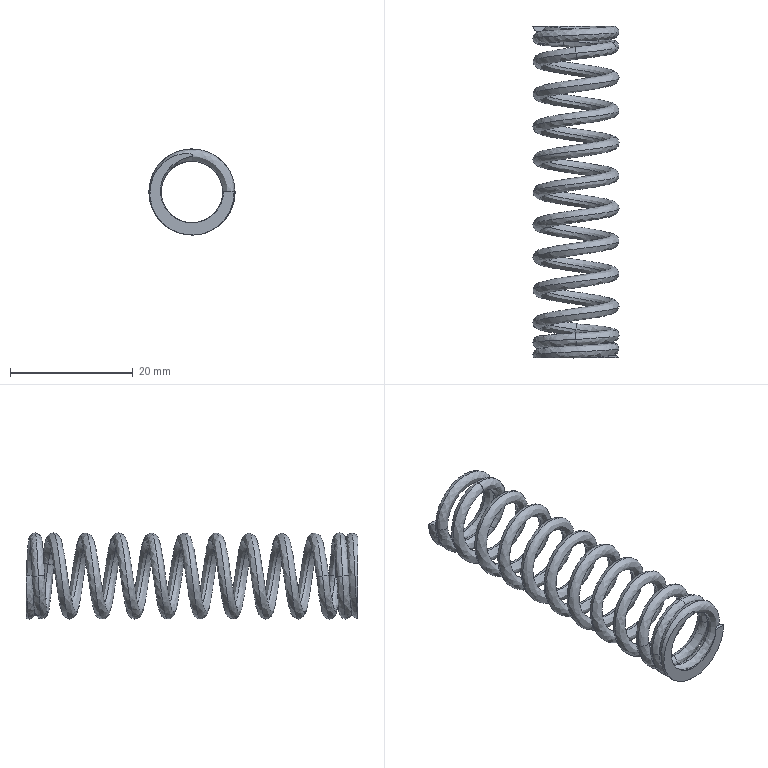Part | STEP file | Compress Spring1 | 1 solid | 26 faces | volume 1385 mm3 | spline 22 | plane 4